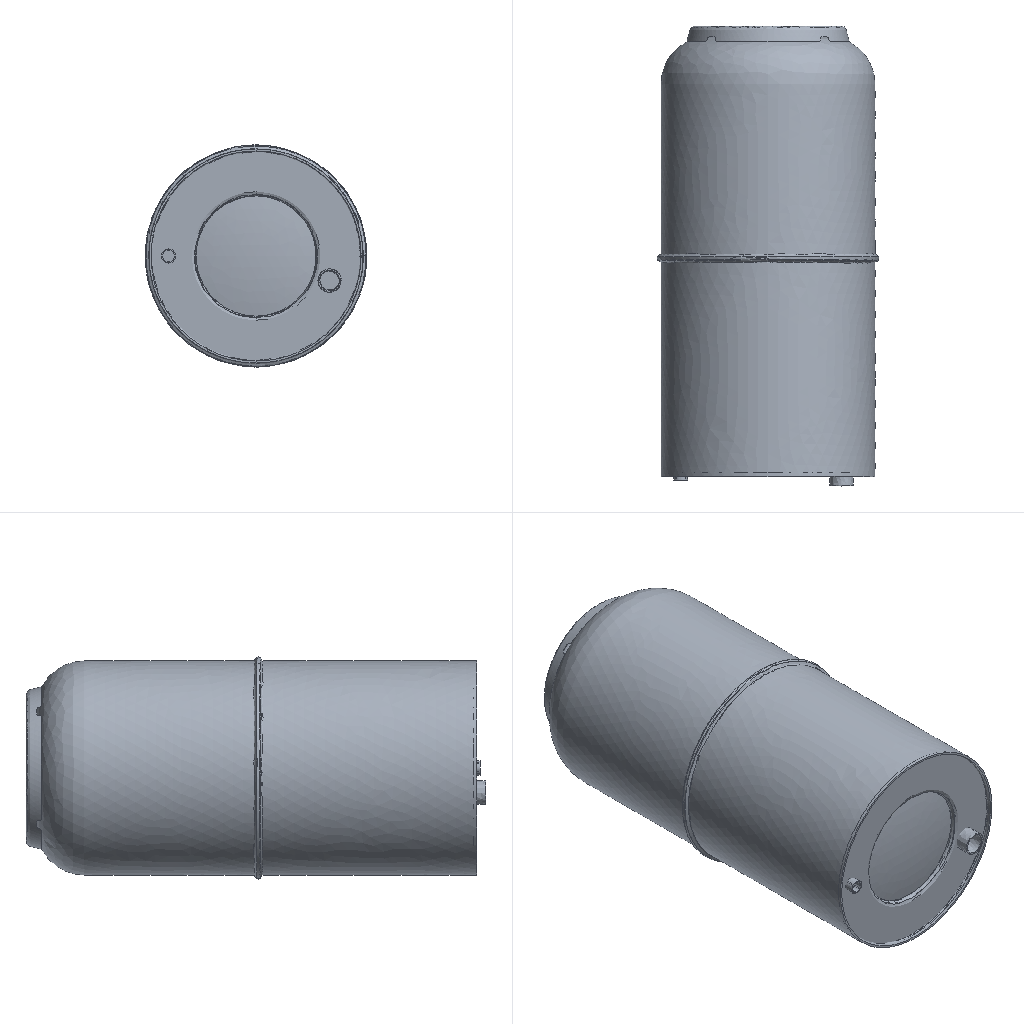Simulation study | ansys workbench
Set-up summary:
category,name,step,type,value,unit,region
solver,ansys_workbench
units,mm-N-s-tonne (MPa),,stated,"/units,MPA"
analysis,deck-1/LS1,,steady-state thermal
load_step,deck-1/LS1,deck-1/LS1,steady-state thermal,nsubst=1; time=4320
load_step,deck-1/LS2,deck-1/LS2,steady-state thermal,nsubst=1; time=8640
load_step,deck-1/LS3,deck-1/LS3,steady-state thermal,nsubst=1; time=12960
load_step,deck-1/LS4,deck-1/LS4,steady-state thermal,nsubst=1; time=17280
load_step,deck-1/LS5,deck-1/LS5,steady-state thermal,nsubst=1; time=21600
load_step,deck-1/LS6,deck-1/LS6,steady-state thermal,nsubst=1; time=25920
load_step,deck-1/LS7,deck-1/LS7,steady-state thermal,nsubst=1; time=30240
load_step,deck-1/LS8,deck-1/LS8,steady-state thermal,nsubst=1; time=34560
load_step,deck-1/LS9,deck-1/LS9,steady-state thermal,nsubst=1; time=38880
load_step,deck-1/LS10,deck-1/LS10,steady-state thermal,nsubst=1; time=43200
load_step,deck-1/LS11,deck-1/LS11,steady-state thermal,nsubst=1; time=47520
load_step,deck-1/LS12,deck-1/LS12,steady-state thermal,nsubst=1; time=51840
load_step,deck-1/LS13,deck-1/LS13,steady-state thermal,nsubst=1; time=56160
load_step,deck-1/LS14,deck-1/LS14,steady-state thermal,nsubst=1; time=60480
load_step,deck-1/LS15,deck-1/LS15,steady-state thermal,nsubst=1; time=64800
load_step,deck-1/LS16,deck-1/LS16,steady-state thermal,nsubst=1; time=69120
load_step,deck-1/LS17,deck-1/LS17,steady-state thermal,nsubst=1; time=73440
load_step,deck-1/LS18,deck-1/LS18,steady-state thermal,nsubst=1; time=77760
load_step,deck-1/LS19,deck-1/LS19,steady-state thermal,nsubst=1; time=82080
load_step,deck-1/LS20,deck-1/LS20,steady-state thermal,nsubst=1; time=86400
analysis,deck-2/LS1,,transient thermal
load_step,deck-2/LS1,deck-2/LS1,transient thermal,nsubst=100; time=0.1
load_step,deck-2/LS2,deck-2/LS2,transient thermal,nsubst=100; time=43200
load_step,deck-2/LS3,deck-2/LS3,transient thermal,nsubst=100; time=86400
mesh,deck-1.dat,,nodes,101538
mesh,deck-1.dat,,elements,67801
element_type,SOLID291,,,49814,,deck-1.dat
element_type,SURF152,,,16555,,deck-1.dat
element_type,TARGE170,,,638,,deck-1.dat
element_type,CONTA174,,,638,,deck-1.dat
element_type,SOLID279,,,156,,deck-1.dat
mesh,deck-2.dat,,nodes,101538
mesh,deck-2.dat,,elements,64700
element_type,SOLID291,,,49814,,deck-2.dat
element_type,SURF152,,,13454,,deck-2.dat
element_type,TARGE170,,,638,,deck-2.dat
element_type,CONTA174,,,638,,deck-2.dat
element_type,SOLID279,,,156,,deck-2.dat
material,304?,,E,193000,tonne s^-2 mm^-1
material,304?,,nu,0.31
material,304?,,density,7.75e-09,tonne mm^-3
material,304?,,conductivity,15.1,tonne mm s^-3 C^-1
material,304?,,specific_heat,4.8e+08,mm^2 s^-2 C^-1
material,304?,,cte,1.7e-05,C^-1
material,304?,,permeability,1
material,304?,,resistivity,0.00077,ohm mm
load,Define Uniform Initial temperature,deck-1/model,body load temp,22,,all
load,"Create ""______""",deck-1/LS1,convection,200000,,SURF152 #16
load,Define Uniform Initial temperature,deck-2/model,body load temp,96,,all
load,"Create ""______""",deck-2/LS1,convection,2.8e-05,,SURF152 #16
load,"Create ""_______________""",deck-2/LS1,convection,1e-07,,SURF152 #17
bc,,deck-1/LS1,temperature,96 [dofs=TEMP n=2],,node list
bc,,deck-2/LS1,temperature,96 [dofs=TEMP],,node list
contact,Contact Region,,bonded (always),element=CONTA174
contact,Contact Region 2,,bonded (always),element=CONTA174
contact,Contact Region 3,,bonded (always),element=CONTA174
contact,Contact Region 4,,bonded (always),element=CONTA174
contact,Contact Region 5,,bonded (always),element=CONTA174
contact,Contact Region,,bonded (always),element=CONTA174
contact,Contact Region 2,,bonded (always),element=CONTA174
contact,Contact Region 3,,bonded (always),element=CONTA174
contact,Contact Region 4,,bonded (always),element=CONTA174
contact,Contact Region 5,,bonded (always),element=CONTA174
named_set,_CM65,,node,11826
named_set,_CM65,,node,10039
Results summary, first 86 of 108 lines:
result,analyses[0].index,,,1
result,analyses[0].system,,,SYS
result,analyses[0].deck,,,deck-1.dat
result,analyses[0].solve_status,,,completed
result,analyses[0].analysis_type,,,static
result,analyses[0].physics,,,thermal
result,analyses[0].unit_system,,,"NMM: mm, ton, N, s, mV, mA, degC"
result,analyses[0].n_sets,,,20
result,analyses[0].load_steps[0].set,set=1,,1
result,analyses[0].load_steps[0].time_or_freq,set=1,,4320
result,analyses[0].load_steps[0].max_temperature,set=1,,98.97
result,analyses[0].load_steps[0].min_temperature,set=1,,17.766
result,analyses[0].load_steps[1].set,set=2,,2
result,analyses[0].load_steps[1].time_or_freq,set=2,,8640
result,analyses[0].load_steps[1].max_temperature,set=2,,98.97
result,analyses[0].load_steps[1].min_temperature,set=2,,17.766
result,analyses[0].load_steps[2].set,set=3,,3
result,analyses[0].load_steps[2].time_or_freq,set=3,,12960
result,analyses[0].load_steps[2].max_temperature,set=3,,98.97
result,analyses[0].load_steps[2].min_temperature,set=3,,17.766
result,analyses[0].load_steps[3].set,set=4,,4
result,analyses[0].load_steps[3].time_or_freq,set=4,,17280
result,analyses[0].load_steps[3].max_temperature,set=4,,98.97
result,analyses[0].load_steps[3].min_temperature,set=4,,17.766
result,analyses[0].load_steps[4].set,set=5,,5
result,analyses[0].load_steps[4].time_or_freq,set=5,,21600
result,analyses[0].load_steps[4].max_temperature,set=5,,98.97
result,analyses[0].load_steps[4].min_temperature,set=5,,17.766
result,analyses[0].load_steps[5].set,set=6,,6
result,analyses[0].load_steps[5].time_or_freq,set=6,,25920
result,analyses[0].load_steps[5].max_temperature,set=6,,98.97
result,analyses[0].load_steps[5].min_temperature,set=6,,17.766
result,analyses[0].load_steps[6].set,set=7,,7
result,analyses[0].load_steps[6].time_or_freq,set=7,,30240
result,analyses[0].load_steps[6].max_temperature,set=7,,98.97
result,analyses[0].load_steps[6].min_temperature,set=7,,17.766
result,analyses[0].load_steps[7].set,set=8,,8
result,analyses[0].load_steps[7].time_or_freq,set=8,,34560
result,analyses[0].load_steps[7].max_temperature,set=8,,98.97
result,analyses[0].load_steps[7].min_temperature,set=8,,17.766
result,analyses[0].load_steps[8].set,set=9,,9
result,analyses[0].load_steps[8].time_or_freq,set=9,,38880
result,analyses[0].load_steps[8].max_temperature,set=9,,98.97
result,analyses[0].load_steps[8].min_temperature,set=9,,17.766
result,analyses[0].load_steps[9].set,set=10,,10
result,analyses[0].load_steps[9].time_or_freq,set=10,,43200
result,analyses[0].load_steps[9].max_temperature,set=10,,98.97
result,analyses[0].load_steps[9].min_temperature,set=10,,17.766
result,analyses[0].load_steps[10].set,set=11,,11
result,analyses[0].load_steps[10].time_or_freq,set=11,,47520
result,analyses[0].load_steps[10].max_temperature,set=11,,98.97
result,analyses[0].load_steps[10].min_temperature,set=11,,17.766
result,analyses[0].load_steps[11].set,set=12,,12
result,analyses[0].load_steps[11].time_or_freq,set=12,,51840
result,analyses[0].load_steps[11].max_temperature,set=12,,98.97
result,analyses[0].load_steps[11].min_temperature,set=12,,17.766
result,analyses[0].load_steps[12].set,set=13,,13
result,analyses[0].load_steps[12].time_or_freq,set=13,,56160
result,analyses[0].load_steps[12].max_temperature,set=13,,98.97
result,analyses[0].load_steps[12].min_temperature,set=13,,17.766
result,analyses[0].load_steps[13].set,set=14,,14
result,analyses[0].load_steps[13].time_or_freq,set=14,,60480
result,analyses[0].load_steps[13].max_temperature,set=14,,98.97
result,analyses[0].load_steps[13].min_temperature,set=14,,17.766
result,analyses[0].load_steps[14].set,set=15,,15
result,analyses[0].load_steps[14].time_or_freq,set=15,,64800
result,analyses[0].load_steps[14].max_temperature,set=15,,98.97
result,analyses[0].load_steps[14].min_temperature,set=15,,17.766
result,analyses[0].load_steps[15].set,set=16,,16
result,analyses[0].load_steps[15].time_or_freq,set=16,,69120
result,analyses[0].load_steps[15].max_temperature,set=16,,98.97
result,analyses[0].load_steps[15].min_temperature,set=16,,17.766
result,analyses[0].load_steps[16].set,set=17,,17
result,analyses[0].load_steps[16].time_or_freq,set=17,,73440
result,analyses[0].load_steps[16].max_temperature,set=17,,98.97
result,analyses[0].load_steps[16].min_temperature,set=17,,17.766
result,analyses[0].load_steps[17].set,set=18,,18
result,analyses[0].load_steps[17].time_or_freq,set=18,,77760
result,analyses[0].load_steps[17].max_temperature,set=18,,98.97
result,analyses[0].load_steps[17].min_temperature,set=18,,17.766
result,analyses[0].load_steps[18].set,set=19,,19
result,analyses[0].load_steps[18].time_or_freq,set=19,,82080
result,analyses[0].load_steps[18].max_temperature,set=19,,98.97
result,analyses[0].load_steps[18].min_temperature,set=19,,17.766
result,analyses[0].load_steps[19].set,set=20,,20
result,analyses[0].load_steps[19].time_or_freq,set=20,,86400